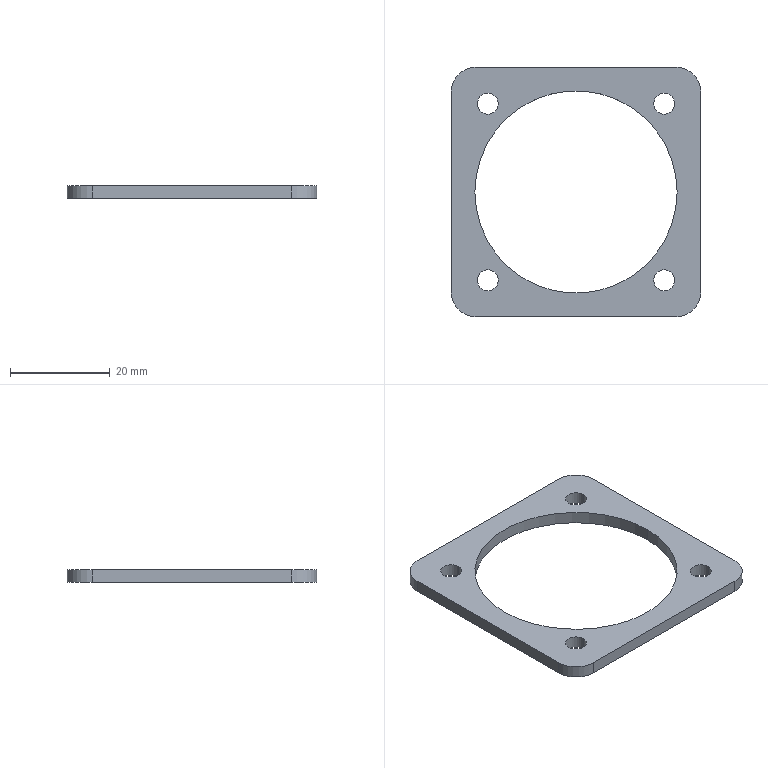Part | SolidWorks | features BaseBody 1 | 1 solid | 20 faces | box 50 x 50 x 2.5 mm | volume 2837 mm3 | cylinder 14 | plane 6 | commonest cylinder face diameters 4.2 x8 10 x4 40.5 x2
STEP:
#1=CARTESIAN_POINT('',(-19.778,17.678,0.));
#2=VERTEX_POINT('',#1);
#3=CARTESIAN_POINT('',(-19.778,17.678,2.5));
#4=VERTEX_POINT('',#3);
#5=CARTESIAN_POINT('',(-19.778,17.678,2.5));
#6=DIRECTION('',(0.,0.,1.));
#7=VECTOR('',#6,1000.);
#8=LINE('',#5,#7);
#9=EDGE_CURVE('',#2,#4,#8,.T.);
#10=ORIENTED_EDGE('',*,*,#9,.F.);
#11=CARTESIAN_POINT('',(-15.578,17.678,0.));
#12=VERTEX_POINT('',#11);
#13=CARTESIAN_POINT('',(-17.678,17.678,0.));
#14=DIRECTION('',(0.,0.,1.));
#15=DIRECTION('',(1.,0.,0.));
#16=AXIS2_PLACEMENT_3D('',#13,#14,#15);
#17=CIRCLE('',#16,2.1);
#18=EDGE_CURVE('',#12,#2,#17,.T.);
#19=ORIENTED_EDGE('',*,*,#18,.F.);
#20=CARTESIAN_POINT('',(-15.578,17.678,2.5));
#21=VERTEX_POINT('',#20);
#22=CARTESIAN_POINT('',(-15.578,17.678,2.5));
#23=DIRECTION('',(0.,0.,1.));
#24=VECTOR('',#23,1000.);
#25=LINE('',#22,#24);
#26=EDGE_CURVE('',#12,#21,#25,.T.);
#27=ORIENTED_EDGE('',*,*,#26,.T.);
#28=CARTESIAN_POINT('',(-17.678,17.678,2.5));
#29=DIRECTION('',(0.,0.,1.));
#30=DIRECTION('',(1.,0.,0.));
#31=AXIS2_PLACEMENT_3D('',#28,#29,#30);
#32=CIRCLE('',#31,2.1);
#33=EDGE_CURVE('',#21,#4,#32,.T.);
#34=ORIENTED_EDGE('',*,*,#33,.T.);
#35=EDGE_LOOP('',(#10,#19,#27,#34));
#36=FACE_OUTER_BOUND('',#35,.T.);
#37=CARTESIAN_POINT('',(-17.678,17.678,2.5));
#38=DIRECTION('',(0.,0.,1.));
#39=DIRECTION('',(1.,0.,0.));
#40=AXIS2_PLACEMENT_3D('',#37,#38,#39);
#41=CYLINDRICAL_SURFACE('',#40,2.1);
#42=ADVANCED_FACE('',(#36),#41,.F.);
#43=CARTESIAN_POINT('',(-19.778,-17.678,0.));
#44=VERTEX_POINT('',#43);
#45=CARTESIAN_POINT('',(-19.778,-17.678,2.5));
#46=VERTEX_POINT('',#45);
#47=CARTESIAN_POINT('',(-19.778,-17.678,2.5));
#48=DIRECTION('',(0.,0.,1.));
#49=VECTOR('',#48,1000.);
#50=LINE('',#47,#49);
#51=EDGE_CURVE('',#44,#46,#50,.T.);
#52=ORIENTED_EDGE('',*,*,#51,.F.);
#53=CARTESIAN_POINT('',(-15.578,-17.678,0.));
#54=VERTEX_POINT('',#53);
#55=CARTESIAN_POINT('',(-17.678,-17.678,0.));
#56=DIRECTION('',(0.,0.,1.));
#57=DIRECTION('',(1.,0.,0.));
#58=AXIS2_PLACEMENT_3D('',#55,#56,#57);
#59=CIRCLE('',#58,2.1);
#60=EDGE_CURVE('',#54,#44,#59,.T.);
#61=ORIENTED_EDGE('',*,*,#60,.F.);
#62=CARTESIAN_POINT('',(-15.578,-17.678,2.5));
#63=VERTEX_POINT('',#62);
#64=CARTESIAN_POINT('',(-15.578,-17.678,2.5));
#65=DIRECTION('',(0.,0.,1.));
#66=VECTOR('',#65,1000.);
#67=LINE('',#64,#66);
#68=EDGE_CURVE('',#54,#63,#67,.T.);
#69=ORIENTED_EDGE('',*,*,#68,.T.);
#70=CARTESIAN_POINT('',(-17.678,-17.678,2.5));
#71=DIRECTION('',(0.,0.,1.));
#72=DIRECTION('',(1.,0.,0.));
#73=AXIS2_PLACEMENT_3D('',#70,#71,#72);
#74=CIRCLE('',#73,2.1);
#75=EDGE_CURVE('',#63,#46,#74,.T.);
#76=ORIENTED_EDGE('',*,*,#75,.T.);
#77=EDGE_LOOP('',(#52,#61,#69,#76));
#78=FACE_OUTER_BOUND('',#77,.T.);
#79=CARTESIAN_POINT('',(-17.678,-17.678,2.5));
#80=DIRECTION('',(0.,0.,1.));
#81=DIRECTION('',(1.,0.,0.));
#82=AXIS2_PLACEMENT_3D('',#79,#80,#81);
#83=CYLINDRICAL_SURFACE('',#82,2.1);
#84=ADVANCED_FACE('',(#78),#83,.F.);
#85=CARTESIAN_POINT('',(15.578,-17.678,0.));
#86=VERTEX_POINT('',#85);
#87=CARTESIAN_POINT('',(15.578,-17.678,2.5));
#88=VERTEX_POINT('',#87);
#89=CARTESIAN_POINT('',(15.578,-17.678,2.5));
#90=DIRECTION('',(0.,0.,1.));
#91=VECTOR('',#90,1000.);
#92=LINE('',#89,#91);
#93=EDGE_CURVE('',#86,#88,#92,.T.);
#94=ORIENTED_EDGE('',*,*,#93,.F.);
#95=CARTESIAN_POINT('',(19.778,-17.678,0.));
#96=VERTEX_POINT('',#95);
#97=CARTESIAN_POINT('',(17.678,-17.678,0.));
#98=DIRECTION('',(0.,0.,1.));
#99=DIRECTION('',(1.,0.,0.));
#100=AXIS2_PLACEMENT_3D('',#97,#98,#99);
#101=CIRCLE('',#100,2.1);
#102=EDGE_CURVE('',#96,#86,#101,.T.);
#103=ORIENTED_EDGE('',*,*,#102,.F.);
#104=CARTESIAN_POINT('',(19.778,-17.678,2.5));
#105=VERTEX_POINT('',#104);
#106=CARTESIAN_POINT('',(19.778,-17.678,2.5));
#107=DIRECTION('',(0.,0.,1.));
#108=VECTOR('',#107,1000.);
#109=LINE('',#106,#108);
#110=EDGE_CURVE('',#96,#105,#109,.T.);
#111=ORIENTED_EDGE('',*,*,#110,.T.);
#112=CARTESIAN_POINT('',(17.678,-17.678,2.5));
#113=DIRECTION('',(0.,0.,1.));
#114=DIRECTION('',(1.,0.,0.));
#115=AXIS2_PLACEMENT_3D('',#112,#113,#114);
#116=CIRCLE('',#115,2.1);
#117=EDGE_CURVE('',#105,#88,#116,.T.);
#118=ORIENTED_EDGE('',*,*,#117,.T.);
#119=EDGE_LOOP('',(#94,#103,#111,#118));
#120=FACE_OUTER_BOUND('',#119,.T.);
#121=CARTESIAN_POINT('',(17.678,-17.678,2.5));
#122=DIRECTION('',(0.,0.,1.));
#123=DIRECTION('',(1.,0.,0.));
#124=AXIS2_PLACEMENT_3D('',#121,#122,#123);
#125=CYLINDRICAL_SURFACE('',#124,2.1);
#126=ADVANCED_FACE('',(#120),#125,.F.);
#127=CARTESIAN_POINT('',(15.578,17.678,0.));
#128=VERTEX_POINT('',#127);
#129=CARTESIAN_POINT('',(15.578,17.678,2.5));
#130=VERTEX_POINT('',#129);
#131=CARTESIAN_POINT('',(15.578,17.678,2.5));
#132=DIRECTION('',(0.,0.,1.));
#133=VECTOR('',#132,1000.);
#134=LINE('',#131,#133);
#135=EDGE_CURVE('',#128,#130,#134,.T.);
#136=ORIENTED_EDGE('',*,*,#135,.F.);
#137=CARTESIAN_POINT('',(19.778,17.678,0.));
#138=VERTEX_POINT('',#137);
#139=CARTESIAN_POINT('',(17.678,17.678,0.));
#140=DIRECTION('',(0.,0.,1.));
#141=DIRECTION('',(1.,0.,0.));
#142=AXIS2_PLACEMENT_3D('',#139,#140,#141);
#143=CIRCLE('',#142,2.1);
#144=EDGE_CURVE('',#138,#128,#143,.T.);
#145=ORIENTED_EDGE('',*,*,#144,.F.);
#146=CARTESIAN_POINT('',(19.778,17.678,2.5));
#147=VERTEX_POINT('',#146);
#148=CARTESIAN_POINT('',(19.778,17.678,2.5));
#149=DIRECTION('',(0.,0.,1.));
#150=VECTOR('',#149,1000.);
#151=LINE('',#148,#150);
#152=EDGE_CURVE('',#138,#147,#151,.T.);
#153=ORIENTED_EDGE('',*,*,#152,.T.);
#154=CARTESIAN_POINT('',(17.678,17.678,2.5));
#155=DIRECTION('',(0.,0.,1.));
#156=DIRECTION('',(1.,0.,0.));
#157=AXIS2_PLACEMENT_3D('',#154,#155,#156);
#158=CIRCLE('',#157,2.1);
#159=EDGE_CURVE('',#147,#130,#158,.T.);
#160=ORIENTED_EDGE('',*,*,#159,.T.);
#161=EDGE_LOOP('',(#136,#145,#153,#160));
#162=FACE_OUTER_BOUND('',#161,.T.);
#163=CARTESIAN_POINT('',(17.678,17.678,2.5));
#164=DIRECTION('',(0.,0.,1.));
#165=DIRECTION('',(1.,0.,0.));
#166=AXIS2_PLACEMENT_3D('',#163,#164,#165);
#167=CYLINDRICAL_SURFACE('',#166,2.1);
#168=ADVANCED_FACE('',(#162),#167,.F.);
#169=CARTESIAN_POINT('',(20.,-25.,2.5));
#170=VERTEX_POINT('',#169);
#171=CARTESIAN_POINT('',(25.,-20.,2.5));
#172=VERTEX_POINT('',#171);
#173=CARTESIAN_POINT('',(20.,-20.,2.5));
#174=DIRECTION('',(0.,0.,1.));
#175=DIRECTION('',(-1.,0.,0.));
#176=AXIS2_PLACEMENT_3D('',#173,#174,#175);
#177=CIRCLE('',#176,5.);
#178=EDGE_CURVE('',#170,#172,#177,.T.);
#179=ORIENTED_EDGE('',*,*,#178,.F.);
#180=CARTESIAN_POINT('',(20.,-25.,0.));
#181=VERTEX_POINT('',#180);
#182=CARTESIAN_POINT('',(20.,-25.,2.5));
#183=DIRECTION('',(0.,0.,1.));
#184=VECTOR('',#183,1000.);
#185=LINE('',#182,#184);
#186=EDGE_CURVE('',#181,#170,#185,.T.);
#187=ORIENTED_EDGE('',*,*,#186,.F.);
#188=CARTESIAN_POINT('',(25.,-20.,0.));
#189=VERTEX_POINT('',#188);
#190=CARTESIAN_POINT('',(20.,-20.,0.));
#191=DIRECTION('',(0.,0.,-1.));
#192=DIRECTION('',(-1.,0.,0.));
#193=AXIS2_PLACEMENT_3D('',#190,#191,#192);
#194=CIRCLE('',#193,5.);
#195=EDGE_CURVE('',#189,#181,#194,.T.);
#196=ORIENTED_EDGE('',*,*,#195,.F.);
#197=CARTESIAN_POINT('',(25.,-20.,2.5));
#198=DIRECTION('',(0.,0.,-1.));
#199=VECTOR('',#198,1000.);
#200=LINE('',#197,#199);
#201=EDGE_CURVE('',#172,#189,#200,.T.);
#202=ORIENTED_EDGE('',*,*,#201,.F.);
#203=EDGE_LOOP('',(#179,#187,#196,#202));
#204=FACE_OUTER_BOUND('',#203,.T.);
#205=CARTESIAN_POINT('',(20.,-20.,2.5));
#206=DIRECTION('',(0.,0.,-1.));
#207=DIRECTION('',(-1.,0.,0.));
#208=AXIS2_PLACEMENT_3D('',#205,#206,#207);
#209=CYLINDRICAL_SURFACE('',#208,5.);
#210=ADVANCED_FACE('',(#204),#209,.T.);
#211=CARTESIAN_POINT('',(-25.,-20.,2.5));
#212=VERTEX_POINT('',#211);
#213=CARTESIAN_POINT('',(-20.,-25.,2.5));
#214=VERTEX_POINT('',#213);
#215=CARTESIAN_POINT('',(-20.,-20.,2.5));
#216=DIRECTION('',(0.,0.,1.));
#217=DIRECTION('',(-1.,0.,0.));
#218=AXIS2_PLACEMENT_3D('',#215,#216,#217);
#219=CIRCLE('',#218,5.);
#220=EDGE_CURVE('',#212,#214,#219,.T.);
#221=ORIENTED_EDGE('',*,*,#220,.F.);
#222=CARTESIAN_POINT('',(-25.,-20.,0.));
#223=VERTEX_POINT('',#222);
#224=CARTESIAN_POINT('',(-25.,-20.,2.5));
#225=DIRECTION('',(0.,0.,1.));
#226=VECTOR('',#225,1000.);
#227=LINE('',#224,#226);
#228=EDGE_CURVE('',#223,#212,#227,.T.);
#229=ORIENTED_EDGE('',*,*,#228,.F.);
#230=CARTESIAN_POINT('',(-20.,-25.,0.));
#231=VERTEX_POINT('',#230);
#232=CARTESIAN_POINT('',(-20.,-20.,0.));
#233=DIRECTION('',(0.,0.,-1.));
#234=DIRECTION('',(-1.,0.,0.));
#235=AXIS2_PLACEMENT_3D('',#232,#233,#234);
#236=CIRCLE('',#235,5.);
#237=EDGE_CURVE('',#231,#223,#236,.T.);
#238=ORIENTED_EDGE('',*,*,#237,.F.);
#239=CARTESIAN_POINT('',(-20.,-25.,2.5));
#240=DIRECTION('',(0.,0.,-1.));
#241=VECTOR('',#240,1000.);
#242=LINE('',#239,#241);
#243=EDGE_CURVE('',#214,#231,#242,.T.);
#244=ORIENTED_EDGE('',*,*,#243,.F.);
#245=EDGE_LOOP('',(#221,#229,#238,#244));
#246=FACE_OUTER_BOUND('',#245,.T.);
#247=CARTESIAN_POINT('',(-20.,-20.,2.5));
#248=DIRECTION('',(0.,0.,-1.));
#249=DIRECTION('',(-1.,0.,0.));
#250=AXIS2_PLACEMENT_3D('',#247,#248,#249);
#251=CYLINDRICAL_SURFACE('',#250,5.);
#252=ADVANCED_FACE('',(#246),#251,.T.);
#253=CARTESIAN_POINT('',(-20.,25.,2.5));
#254=VERTEX_POINT('',#253);
#255=CARTESIAN_POINT('',(-25.,20.,2.5));
#256=VERTEX_POINT('',#255);
#257=CARTESIAN_POINT('',(-20.,20.,2.5));
#258=DIRECTION('',(0.,0.,1.));
#259=DIRECTION('',(-1.,0.,0.));
#260=AXIS2_PLACEMENT_3D('',#257,#258,#259);
#261=CIRCLE('',#260,5.);
#262=EDGE_CURVE('',#254,#256,#261,.T.);
#263=ORIENTED_EDGE('',*,*,#262,.F.);
#264=CARTESIAN_POINT('',(-20.,25.,0.));
#265=VERTEX_POINT('',#264);
#266=CARTESIAN_POINT('',(-20.,25.,2.5));
#267=DIRECTION('',(0.,0.,1.));
#268=VECTOR('',#267,1000.);
#269=LINE('',#266,#268);
#270=EDGE_CURVE('',#265,#254,#269,.T.);
#271=ORIENTED_EDGE('',*,*,#270,.F.);
#272=CARTESIAN_POINT('',(-25.,20.,0.));
#273=VERTEX_POINT('',#272);
#274=CARTESIAN_POINT('',(-20.,20.,0.));
#275=DIRECTION('',(0.,0.,-1.));
#276=DIRECTION('',(-1.,0.,0.));
#277=AXIS2_PLACEMENT_3D('',#274,#275,#276);
#278=CIRCLE('',#277,5.);
#279=EDGE_CURVE('',#273,#265,#278,.T.);
#280=ORIENTED_EDGE('',*,*,#279,.F.);
#281=CARTESIAN_POINT('',(-25.,20.,2.5));
#282=DIRECTION('',(0.,0.,-1.));
#283=VECTOR('',#282,1000.);
#284=LINE('',#281,#283);
#285=EDGE_CURVE('',#256,#273,#284,.T.);
#286=ORIENTED_EDGE('',*,*,#285,.F.);
#287=EDGE_LOOP('',(#263,#271,#280,#286));
#288=FACE_OUTER_BOUND('',#287,.T.);
#289=CARTESIAN_POINT('',(-20.,20.,2.5));
#290=DIRECTION('',(0.,0.,-1.));
#291=DIRECTION('',(-1.,0.,0.));
#292=AXIS2_PLACEMENT_3D('',#289,#290,#291);
#293=CYLINDRICAL_SURFACE('',#292,5.);
#294=ADVANCED_FACE('',(#288),#293,.T.);
#295=CARTESIAN_POINT('',(25.,20.,2.5));
#296=VERTEX_POINT('',#295);
#297=CARTESIAN_POINT('',(20.,25.,2.5));
#298=VERTEX_POINT('',#297);
#299=CARTESIAN_POINT('',(20.,20.,2.5));
#300=DIRECTION('',(0.,0.,1.));
#301=DIRECTION('',(-1.,0.,0.));
#302=AXIS2_PLACEMENT_3D('',#299,#300,#301);
#303=CIRCLE('',#302,5.);
#304=EDGE_CURVE('',#296,#298,#303,.T.);
#305=ORIENTED_EDGE('',*,*,#304,.F.);
#306=CARTESIAN_POINT('',(25.,20.,0.));
#307=VERTEX_POINT('',#306);
#308=CARTESIAN_POINT('',(25.,20.,2.5));
#309=DIRECTION('',(0.,0.,1.));
#310=VECTOR('',#309,1000.);
#311=LINE('',#308,#310);
#312=EDGE_CURVE('',#307,#296,#311,.T.);
#313=ORIENTED_EDGE('',*,*,#312,.F.);
#314=CARTESIAN_POINT('',(20.,25.,0.));
#315=VERTEX_POINT('',#314);
#316=CARTESIAN_POINT('',(20.,20.,0.));
#317=DIRECTION('',(0.,0.,-1.));
#318=DIRECTION('',(-1.,0.,0.));
#319=AXIS2_PLACEMENT_3D('',#316,#317,#318);
#320=CIRCLE('',#319,5.);
#321=EDGE_CURVE('',#315,#307,#320,.T.);
#322=ORIENTED_EDGE('',*,*,#321,.F.);
#323=CARTESIAN_POINT('',(20.,25.,2.5));
#324=DIRECTION('',(0.,0.,-1.));
#325=VECTOR('',#324,1000.);
#326=LINE('',#323,#325);
#327=EDGE_CURVE('',#298,#315,#326,.T.);
#328=ORIENTED_EDGE('',*,*,#327,.F.);
#329=EDGE_LOOP('',(#305,#313,#322,#328));
#330=FACE_OUTER_BOUND('',#329,.T.);
#331=CARTESIAN_POINT('',(20.,20.,2.5));
#332=DIRECTION('',(0.,0.,-1.));
#333=DIRECTION('',(-1.,0.,0.));
#334=AXIS2_PLACEMENT_3D('',#331,#332,#333);
#335=CYLINDRICAL_SURFACE('',#334,5.);
#336=ADVANCED_FACE('',(#330),#335,.T.);
#337=CARTESIAN_POINT('',(20.25,0.,2.5));
#338=VERTEX_POINT('',#337);
#339=CARTESIAN_POINT('',(20.25,0.,0.));
#340=VERTEX_POINT('',#339);
#341=CARTESIAN_POINT('',(20.25,0.,2.5));
#342=DIRECTION('',(0.,0.,-1.));
#343=VECTOR('',#342,1000.);
#344=LINE('',#341,#343);
#345=EDGE_CURVE('',#338,#340,#344,.T.);
#346=ORIENTED_EDGE('',*,*,#345,.F.);
#347=CARTESIAN_POINT('',(-20.25,0.,2.5));
#348=VERTEX_POINT('',#347);
#349=CARTESIAN_POINT('',(0.,0.,2.5));
#350=DIRECTION('',(0.,0.,1.));
#351=DIRECTION('',(1.,0.,0.));
#352=AXIS2_PLACEMENT_3D('',#349,#350,#351);
#353=CIRCLE('',#352,20.25);
#354=EDGE_CURVE('',#338,#348,#353,.T.);
#355=ORIENTED_EDGE('',*,*,#354,.T.);
#356=CARTESIAN_POINT('',(-20.25,0.,0.));
#357=VERTEX_POINT('',#356);
#358=CARTESIAN_POINT('',(-20.25,0.,2.5));
#359=DIRECTION('',(0.,0.,-1.));
#360=VECTOR('',#359,1000.);
#361=LINE('',#358,#360);
#362=EDGE_CURVE('',#348,#357,#361,.T.);
#363=ORIENTED_EDGE('',*,*,#362,.T.);
#364=CARTESIAN_POINT('',(0.,0.,0.));
#365=DIRECTION('',(0.,0.,1.));
#366=DIRECTION('',(1.,0.,0.));
#367=AXIS2_PLACEMENT_3D('',#364,#365,#366);
#368=CIRCLE('',#367,20.25);
#369=EDGE_CURVE('',#340,#357,#368,.T.);
#370=ORIENTED_EDGE('',*,*,#369,.F.);
#371=EDGE_LOOP('',(#346,#355,#363,#370));
#372=FACE_OUTER_BOUND('',#371,.T.);
#373=CARTESIAN_POINT('',(0.,0.,2.5));
#374=DIRECTION('',(0.,0.,-1.));
#375=DIRECTION('',(-1.,0.,0.));
#376=AXIS2_PLACEMENT_3D('',#373,#374,#375);
#377=CYLINDRICAL_SURFACE('',#376,20.25);
#378=ADVANCED_FACE('',(#372),#377,.F.);
#379=CARTESIAN_POINT('',(-25.,-25.,2.5));
#380=DIRECTION('',(1.,0.,0.));
#381=VECTOR('',#380,1000.);
#382=LINE('',#379,#381);
#383=EDGE_CURVE('',#214,#170,#382,.T.);
#384=ORIENTED_EDGE('',*,*,#383,.F.);
#385=ORIENTED_EDGE('',*,*,#243,.T.);
#386=CARTESIAN_POINT('',(-25.,-25.,0.));
#387=DIRECTION('',(1.,0.,0.));
#388=VECTOR('',#387,1000.);
#389=LINE('',#386,#388);
#390=EDGE_CURVE('',#231,#181,#389,.T.);
#391=ORIENTED_EDGE('',*,*,#390,.T.);
#392=ORIENTED_EDGE('',*,*,#186,.T.);
#393=EDGE_LOOP('',(#384,#385,#391,#392));
#394=FACE_OUTER_BOUND('',#393,.T.);
#395=CARTESIAN_POINT('',(-25.,-25.,2.5));
#396=DIRECTION('',(0.,1.,0.));
#397=DIRECTION('',(1.,0.,0.));
#398=AXIS2_PLACEMENT_3D('',#395,#396,#397);
#399=PLANE('',#398);
#400=ADVANCED_FACE('',(#394),#399,.F.);
#401=CARTESIAN_POINT('',(-25.,-25.,2.5));
#402=DIRECTION('',(0.,-1.,0.));
#403=VECTOR('',#402,1000.);
#404=LINE('',#401,#403);
#405=EDGE_CURVE('',#256,#212,#404,.T.);
#406=ORIENTED_EDGE('',*,*,#405,.F.);
#407=ORIENTED_EDGE('',*,*,#285,.T.);
#408=CARTESIAN_POINT('',(-25.,-25.,0.));
#409=DIRECTION('',(0.,-1.,0.));
#410=VECTOR('',#409,1000.);
#411=LINE('',#408,#410);
#412=EDGE_CURVE('',#273,#223,#411,.T.);
#413=ORIENTED_EDGE('',*,*,#412,.T.);
#414=ORIENTED_EDGE('',*,*,#228,.T.);
#415=EDGE_LOOP('',(#406,#407,#413,#414));
#416=FACE_OUTER_BOUND('',#415,.T.);
#417=CARTESIAN_POINT('',(-25.,-25.,2.5));
#418=DIRECTION('',(1.,0.,0.));
#419=DIRECTION('',(0.,1.,0.));
#420=AXIS2_PLACEMENT_3D('',#417,#418,#419);
#421=PLANE('',#420);
#422=ADVANCED_FACE('',(#416),#421,.F.);
#423=CARTESIAN_POINT('',(-25.,25.,2.5));
#424=DIRECTION('',(-1.,0.,0.));
#425=VECTOR('',#424,1000.);
#426=LINE('',#423,#425);
#427=EDGE_CURVE('',#298,#254,#426,.T.);
#428=ORIENTED_EDGE('',*,*,#427,.F.);
#429=ORIENTED_EDGE('',*,*,#327,.T.);
#430=CARTESIAN_POINT('',(-25.,25.,0.));
#431=DIRECTION('',(-1.,0.,0.));
#432=VECTOR('',#431,1000.);
#433=LINE('',#430,#432);
#434=EDGE_CURVE('',#315,#265,#433,.T.);
#435=ORIENTED_EDGE('',*,*,#434,.T.);
#436=ORIENTED_EDGE('',*,*,#270,.T.);
#437=EDGE_LOOP('',(#428,#429,#435,#436));
#438=FACE_OUTER_BOUND('',#437,.T.);
#439=CARTESIAN_POINT('',(-25.,25.,2.5));
#440=DIRECTION('',(0.,-1.,0.));
#441=DIRECTION('',(0.,0.,-1.));
#442=AXIS2_PLACEMENT_3D('',#439,#440,#441);
#443=PLANE('',#442);
#444=ADVANCED_FACE('',(#438),#443,.F.);
#445=CARTESIAN_POINT('',(25.,-25.,0.));
#446=DIRECTION('',(0.,1.,0.));
#447=VECTOR('',#446,1000.);
#448=LINE('',#445,#447);
#449=EDGE_CURVE('',#189,#307,#448,.T.);
#450=ORIENTED_EDGE('',*,*,#449,.T.);
#451=ORIENTED_EDGE('',*,*,#312,.T.);
#452=CARTESIAN_POINT('',(25.,-25.,2.5));
#453=DIRECTION('',(0.,1.,0.));
#454=VECTOR('',#453,1000.);
#455=LINE('',#452,#454);
#456=EDGE_CURVE('',#172,#296,#455,.T.);
#457=ORIENTED_EDGE('',*,*,#456,.F.);
#458=ORIENTED_EDGE('',*,*,#201,.T.);
#459=EDGE_LOOP('',(#450,#451,#457,#458));
#460=FACE_OUTER_BOUND('',#459,.T.);
#461=CARTESIAN_POINT('',(25.,-25.,2.5));
#462=DIRECTION('',(-1.,0.,0.));
#463=DIRECTION('',(0.,0.,1.));
#464=AXIS2_PLACEMENT_3D('',#461,#462,#463);
#465=PLANE('',#464);
#466=ADVANCED_FACE('',(#460),#465,.F.);
#467=CARTESIAN_POINT('',(0.,0.,2.5));
#468=DIRECTION('',(0.,0.,1.));
#469=DIRECTION('',(1.,0.,0.));
#470=AXIS2_PLACEMENT_3D('',#467,#468,#469);
#471=CIRCLE('',#470,20.25);
#472=EDGE_CURVE('',#348,#338,#471,.T.);
#473=ORIENTED_EDGE('',*,*,#472,.F.);
#474=ORIENTED_EDGE('',*,*,#354,.F.);
#475=EDGE_LOOP('',(#473,#474));
#476=FACE_BOUND('',#475,.T.);
#477=ORIENTED_EDGE('',*,*,#159,.F.);
#478=CARTESIAN_POINT('',(17.678,17.678,2.5));
#479=DIRECTION('',(0.,0.,1.));
#480=DIRECTION('',(1.,0.,0.));
#481=AXIS2_PLACEMENT_3D('',#478,#479,#480);
#482=CIRCLE('',#481,2.1);
#483=EDGE_CURVE('',#130,#147,#482,.T.);
#484=ORIENTED_EDGE('',*,*,#483,.F.);
#485=EDGE_LOOP('',(#477,#484));
#486=FACE_BOUND('',#485,.T.);
#487=ORIENTED_EDGE('',*,*,#117,.F.);
#488=CARTESIAN_POINT('',(17.678,-17.678,2.5));
#489=DIRECTION('',(0.,0.,1.));
#490=DIRECTION('',(1.,0.,0.));
#491=AXIS2_PLACEMENT_3D('',#488,#489,#490);
#492=CIRCLE('',#491,2.1);
#493=EDGE_CURVE('',#88,#105,#492,.T.);
#494=ORIENTED_EDGE('',*,*,#493,.F.);
#495=EDGE_LOOP('',(#487,#494));
#496=FACE_BOUND('',#495,.T.);
#497=ORIENTED_EDGE('',*,*,#75,.F.);
#498=CARTESIAN_POINT('',(-17.678,-17.678,2.5));
#499=DIRECTION('',(0.,0.,1.));
#500=DIRECTION('',(1.,0.,0.));
#501=AXIS2_PLACEMENT_3D('',#498,#499,#500);
#502=CIRCLE('',#501,2.1);
#503=EDGE_CURVE('',#46,#63,#502,.T.);
#504=ORIENTED_EDGE('',*,*,#503,.F.);
#505=EDGE_LOOP('',(#497,#504));
#506=FACE_BOUND('',#505,.T.);
#507=ORIENTED_EDGE('',*,*,#33,.F.);
#508=CARTESIAN_POINT('',(-17.678,17.678,2.5));
#509=DIRECTION('',(0.,0.,1.));
#510=DIRECTION('',(1.,0.,0.));
#511=AXIS2_PLACEMENT_3D('',#508,#509,#510);
#512=CIRCLE('',#511,2.1);
#513=EDGE_CURVE('',#4,#21,#512,.T.);
#514=ORIENTED_EDGE('',*,*,#513,.F.);
#515=EDGE_LOOP('',(#507,#514));
#516=FACE_BOUND('',#515,.T.);
#517=ORIENTED_EDGE('',*,*,#456,.T.);
#518=ORIENTED_EDGE('',*,*,#304,.T.);
#519=ORIENTED_EDGE('',*,*,#427,.T.);
#520=ORIENTED_EDGE('',*,*,#262,.T.);
#521=ORIENTED_EDGE('',*,*,#405,.T.);
#522=ORIENTED_EDGE('',*,*,#220,.T.);
#523=ORIENTED_EDGE('',*,*,#383,.T.);
#524=ORIENTED_EDGE('',*,*,#178,.T.);
#525=EDGE_LOOP('',(#517,#518,#519,#520,#521,#522,#523,#524));
#526=FACE_OUTER_BOUND('',#525,.T.);
#527=CARTESIAN_POINT('',(0.,0.,2.5));
#528=DIRECTION('',(0.,0.,-1.));
#529=DIRECTION('',(0.,-1.,0.));
#530=AXIS2_PLACEMENT_3D('',#527,#528,#529);
#531=PLANE('',#530);
#532=ADVANCED_FACE('',(#476,#486,#496,#506,#516,#526),#531,.F.);
#533=ORIENTED_EDGE('',*,*,#102,.T.);
#534=CARTESIAN_POINT('',(17.678,-17.678,0.));
#535=DIRECTION('',(0.,0.,1.));
#536=DIRECTION('',(1.,0.,0.));
#537=AXIS2_PLACEMENT_3D('',#534,#535,#536);
#538=CIRCLE('',#537,2.1);
#539=EDGE_CURVE('',#86,#96,#538,.T.);
#540=ORIENTED_EDGE('',*,*,#539,.T.);
#541=EDGE_LOOP('',(#533,#540));
#542=FACE_BOUND('',#541,.T.);
#543=ORIENTED_EDGE('',*,*,#144,.T.);
#544=CARTESIAN_POINT('',(17.678,17.678,0.));
#545=DIRECTION('',(0.,0.,1.));
#546=DIRECTION('',(1.,0.,0.));
#547=AXIS2_PLACEMENT_3D('',#544,#545,#546);
#548=CIRCLE('',#547,2.1);
#549=EDGE_CURVE('',#128,#138,#548,.T.);
#550=ORIENTED_EDGE('',*,*,#549,.T.);
#551=EDGE_LOOP('',(#543,#550));
#552=FACE_BOUND('',#551,.T.);
#553=CARTESIAN_POINT('',(0.,0.,0.));
#554=DIRECTION('',(0.,0.,1.));
#555=DIRECTION('',(1.,0.,0.));
#556=AXIS2_PLACEMENT_3D('',#553,#554,#555);
#557=CIRCLE('',#556,20.25);
#558=EDGE_CURVE('',#357,#340,#557,.T.);
#559=ORIENTED_EDGE('',*,*,#558,.T.);
#560=ORIENTED_EDGE('',*,*,#369,.T.);
#561=EDGE_LOOP('',(#559,#560));
#562=FACE_BOUND('',#561,.T.);
#563=ORIENTED_EDGE('',*,*,#60,.T.);
#564=CARTESIAN_POINT('',(-17.678,-17.678,0.));
#565=DIRECTION('',(0.,0.,1.));
#566=DIRECTION('',(1.,0.,0.));
#567=AXIS2_PLACEMENT_3D('',#564,#565,#566);
#568=CIRCLE('',#567,2.1);
#569=EDGE_CURVE('',#44,#54,#568,.T.);
#570=ORIENTED_EDGE('',*,*,#569,.T.);
#571=EDGE_LOOP('',(#563,#570));
#572=FACE_BOUND('',#571,.T.);
#573=ORIENTED_EDGE('',*,*,#18,.T.);
#574=CARTESIAN_POINT('',(-17.678,17.678,0.));
#575=DIRECTION('',(0.,0.,1.));
#576=DIRECTION('',(1.,0.,0.));
#577=AXIS2_PLACEMENT_3D('',#574,#575,#576);
#578=CIRCLE('',#577,2.1);
#579=EDGE_CURVE('',#2,#12,#578,.T.);
#580=ORIENTED_EDGE('',*,*,#579,.T.);
#581=EDGE_LOOP('',(#573,#580));
#582=FACE_BOUND('',#581,.T.);
#583=ORIENTED_EDGE('',*,*,#434,.F.);
#584=ORIENTED_EDGE('',*,*,#321,.T.);
#585=ORIENTED_EDGE('',*,*,#449,.F.);
#586=ORIENTED_EDGE('',*,*,#195,.T.);
#587=ORIENTED_EDGE('',*,*,#390,.F.);
#588=ORIENTED_EDGE('',*,*,#237,.T.);
#589=ORIENTED_EDGE('',*,*,#412,.F.);
#590=ORIENTED_EDGE('',*,*,#279,.T.);
#591=EDGE_LOOP('',(#583,#584,#585,#586,#587,#588,#589,#590));
#592=FACE_OUTER_BOUND('',#591,.T.);
#593=CARTESIAN_POINT('',(0.,0.,0.));
#594=DIRECTION('',(0.,0.,-1.));
#595=DIRECTION('',(0.,-1.,0.));
#596=AXIS2_PLACEMENT_3D('',#593,#594,#595);
#597=PLANE('',#596);
#598=ADVANCED_FACE('',(#542,#552,#562,#572,#582,#592),#597,.T.);
#599=ORIENTED_EDGE('',*,*,#472,.T.);
#600=ORIENTED_EDGE('',*,*,#345,.T.);
#601=ORIENTED_EDGE('',*,*,#558,.F.);
#602=ORIENTED_EDGE('',*,*,#362,.F.);
#603=EDGE_LOOP('',(#599,#600,#601,#602));
#604=FACE_OUTER_BOUND('',#603,.T.);
#605=CARTESIAN_POINT('',(0.,0.,2.5));
#606=DIRECTION('',(0.,0.,-1.));
#607=DIRECTION('',(-1.,0.,0.));
#608=AXIS2_PLACEMENT_3D('',#605,#606,#607);
#609=CYLINDRICAL_SURFACE('',#608,20.25);
#610=ADVANCED_FACE('',(#604),#609,.F.);
#611=ORIENTED_EDGE('',*,*,#549,.F.);
#612=ORIENTED_EDGE('',*,*,#135,.T.);
#613=ORIENTED_EDGE('',*,*,#483,.T.);
#614=ORIENTED_EDGE('',*,*,#152,.F.);
#615=EDGE_LOOP('',(#611,#612,#613,#614));
#616=FACE_OUTER_BOUND('',#615,.T.);
#617=CARTESIAN_POINT('',(17.678,17.678,2.5));
#618=DIRECTION('',(0.,0.,1.));
#619=DIRECTION('',(1.,0.,0.));
#620=AXIS2_PLACEMENT_3D('',#617,#618,#619);
#621=CYLINDRICAL_SURFACE('',#620,2.1);
#622=ADVANCED_FACE('',(#616),#621,.F.);
#623=ORIENTED_EDGE('',*,*,#539,.F.);
#624=ORIENTED_EDGE('',*,*,#93,.T.);
#625=ORIENTED_EDGE('',*,*,#493,.T.);
#626=ORIENTED_EDGE('',*,*,#110,.F.);
#627=EDGE_LOOP('',(#623,#624,#625,#626));
#628=FACE_OUTER_BOUND('',#627,.T.);
#629=CARTESIAN_POINT('',(17.678,-17.678,2.5));
#630=DIRECTION('',(0.,0.,1.));
#631=DIRECTION('',(1.,0.,0.));
#632=AXIS2_PLACEMENT_3D('',#629,#630,#631);
#633=CYLINDRICAL_SURFACE('',#632,2.1);
#634=ADVANCED_FACE('',(#628),#633,.F.);
#635=ORIENTED_EDGE('',*,*,#569,.F.);
#636=ORIENTED_EDGE('',*,*,#51,.T.);
#637=ORIENTED_EDGE('',*,*,#503,.T.);
#638=ORIENTED_EDGE('',*,*,#68,.F.);
#639=EDGE_LOOP('',(#635,#636,#637,#638));
#640=FACE_OUTER_BOUND('',#639,.T.);
#641=CARTESIAN_POINT('',(-17.678,-17.678,2.5));
#642=DIRECTION('',(0.,0.,1.));
#643=DIRECTION('',(1.,0.,0.));
#644=AXIS2_PLACEMENT_3D('',#641,#642,#643);
#645=CYLINDRICAL_SURFACE('',#644,2.1);
#646=ADVANCED_FACE('',(#640),#645,.F.);
#647=ORIENTED_EDGE('',*,*,#579,.F.);
#648=ORIENTED_EDGE('',*,*,#9,.T.);
#649=ORIENTED_EDGE('',*,*,#513,.T.);
#650=ORIENTED_EDGE('',*,*,#26,.F.);
#651=EDGE_LOOP('',(#647,#648,#649,#650));
#652=FACE_OUTER_BOUND('',#651,.T.);
#653=CARTESIAN_POINT('',(-17.678,17.678,2.5));
#654=DIRECTION('',(0.,0.,1.));
#655=DIRECTION('',(1.,0.,0.));
#656=AXIS2_PLACEMENT_3D('',#653,#654,#655);
#657=CYLINDRICAL_SURFACE('',#656,2.1);
#658=ADVANCED_FACE('',(#652),#657,.F.);
#659=CLOSED_SHELL('',(#42,#84,#126,#168,#210,#252,#294,#336,#378,#400,#422,#444,#466,#532,#598,#610,#622,#634,#646,#658));
#660=MANIFOLD_SOLID_BREP('',#659);
#661=CARTESIAN_POINT('',(0.,0.,0.));
#662=DIRECTION('',(0.,0.,1.));
#663=DIRECTION('',(1.,0.,0.));
#664=AXIS2_PLACEMENT_3D('',#661,#662,#663);
#665=(LENGTH_UNIT()NAMED_UNIT(*)SI_UNIT(.MILLI.,.METRE.));
#666=UNCERTAINTY_MEASURE_WITH_UNIT(LENGTH_MEASURE(0.00001),#665,'','');
#667=(NAMED_UNIT(*)PLANE_ANGLE_UNIT()SI_UNIT($,.RADIAN.));
#668=(NAMED_UNIT(*)SI_UNIT($,.STERADIAN.)SOLID_ANGLE_UNIT());
#669=(GEOMETRIC_REPRESENTATION_CONTEXT(3)GLOBAL_UNCERTAINTY_ASSIGNED_CONTEXT((#666))GLOBAL_UNIT_ASSIGNED_CONTEXT((#665,#667,#668))REPRESENTATION_CONTEXT('',''));
#670=ADVANCED_BREP_SHAPE_REPRESENTATION('',(#660,#664),#669);